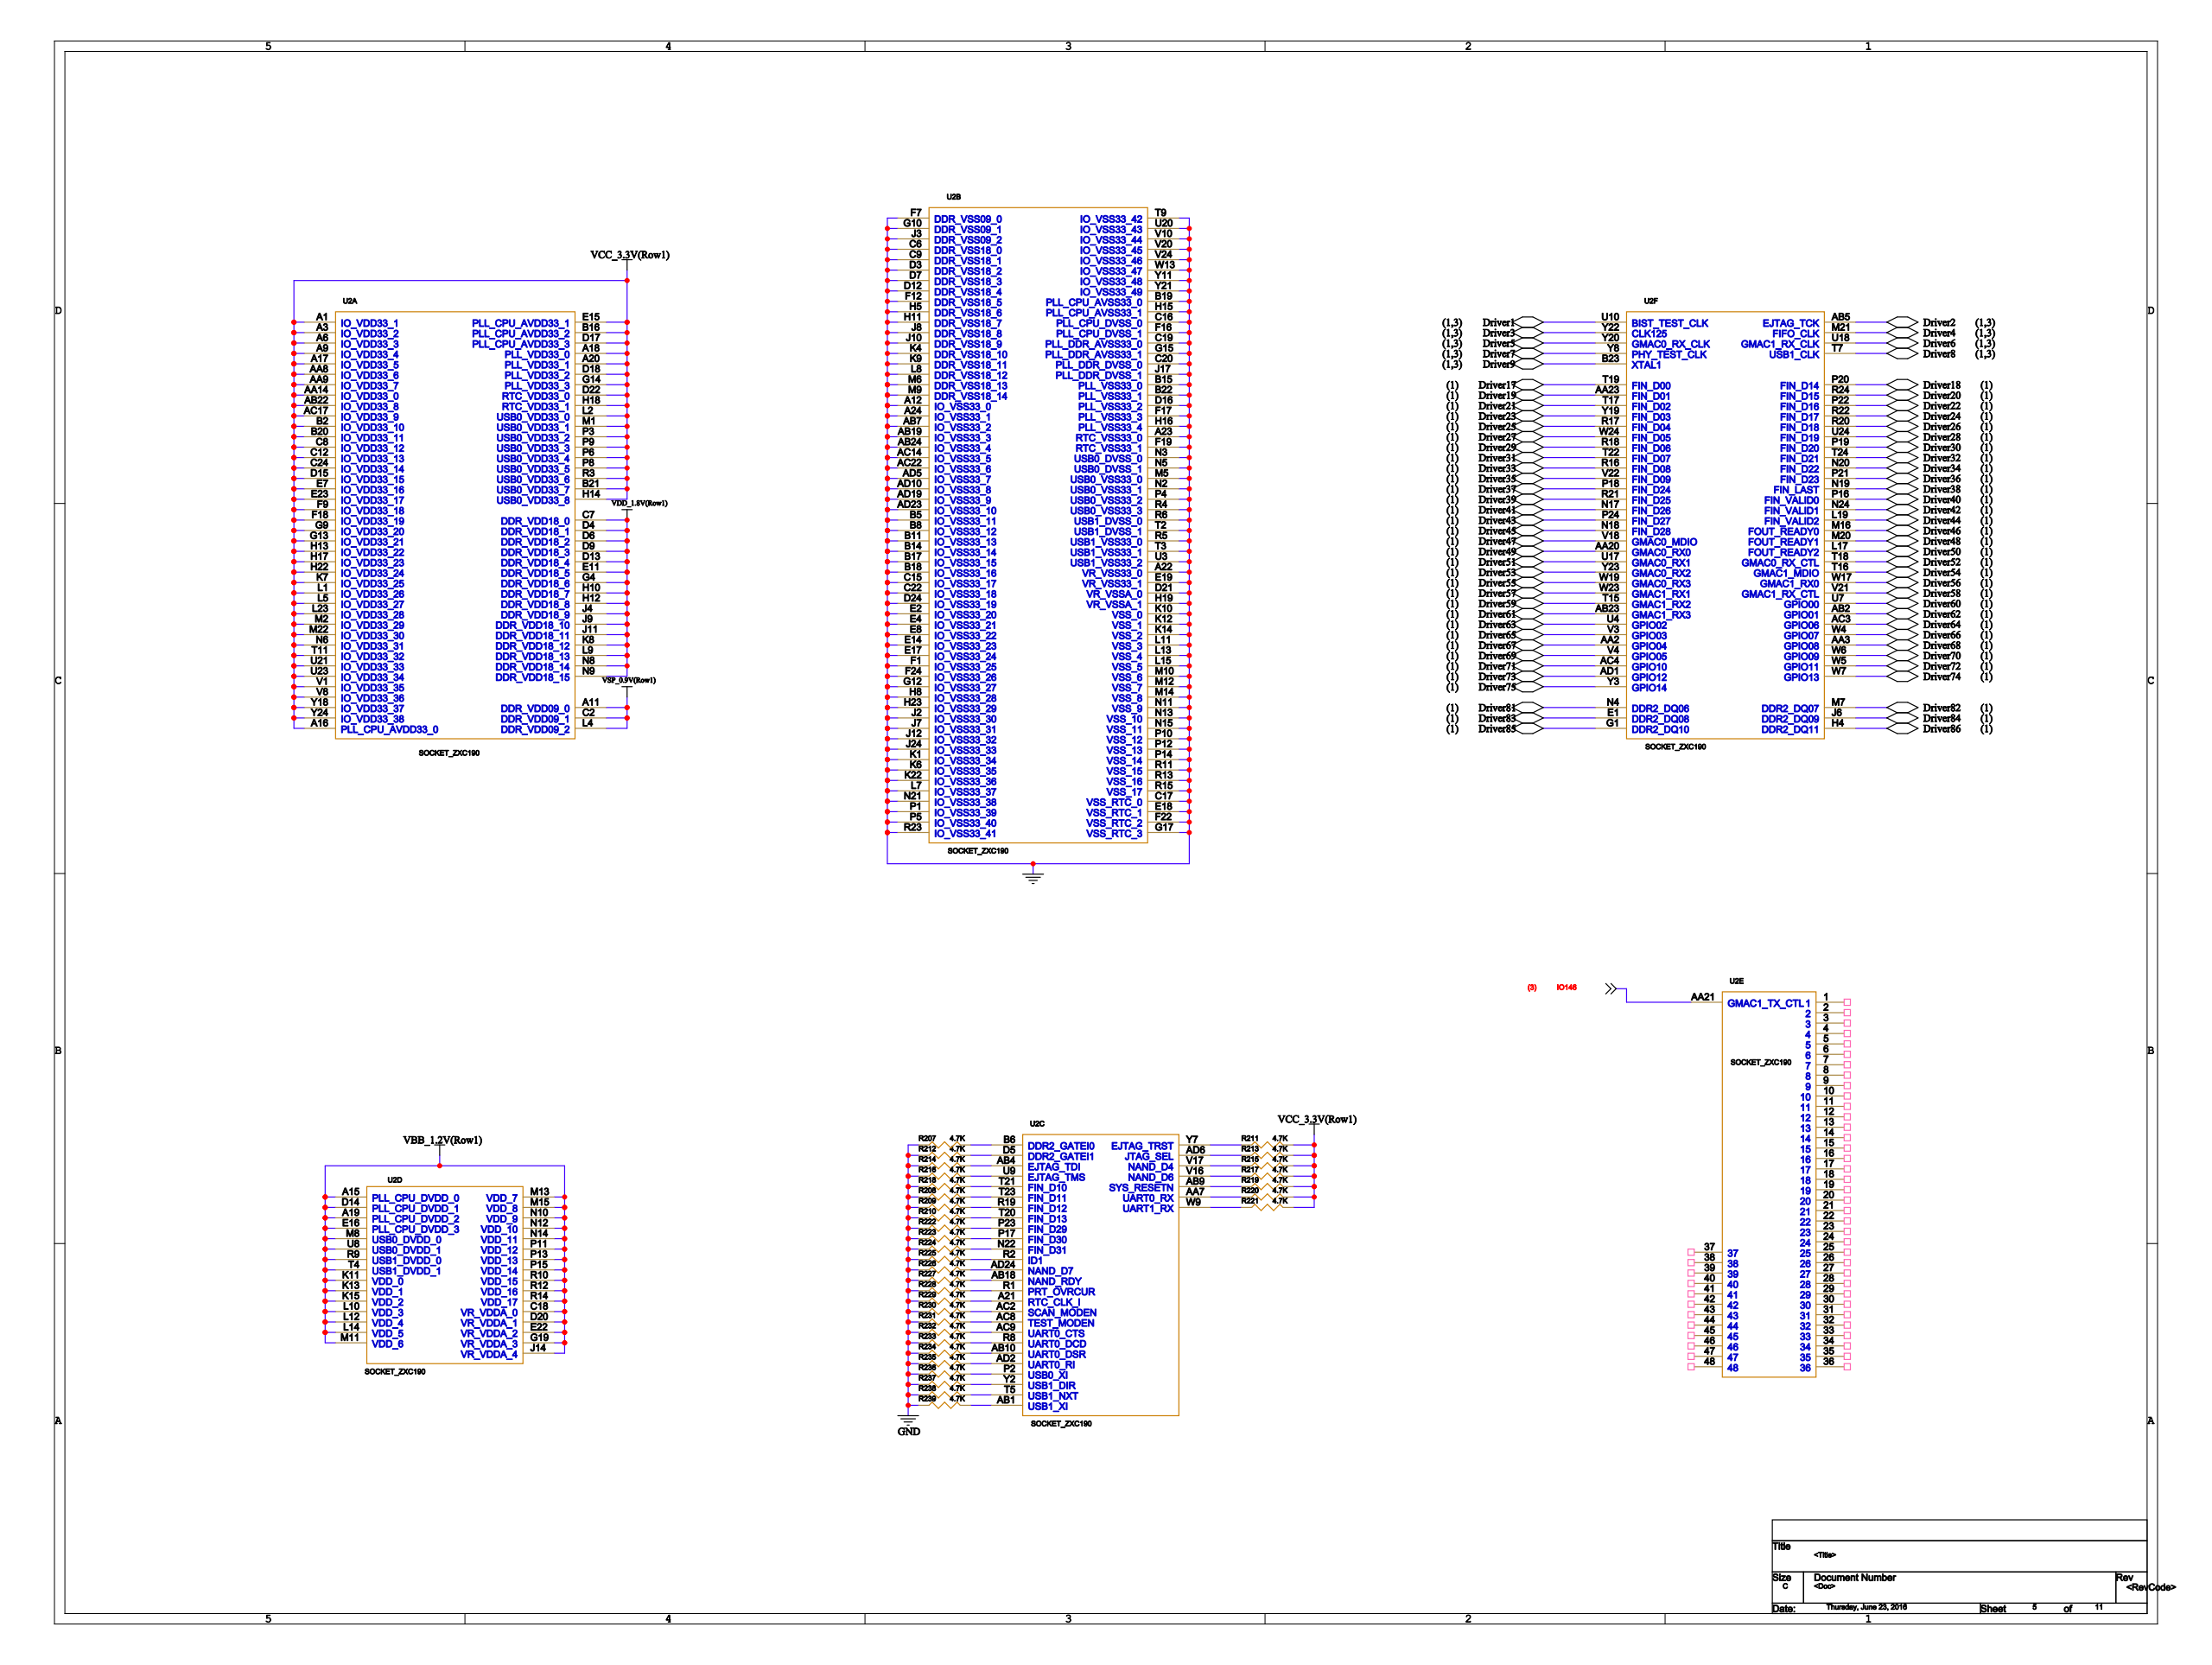Circuit board | Cadence Allegro | 531 parts | 624 nets | one sheet of the schematic
Parts on this sheet (reference | value | footprint):
R207 | 4.7K | R0805
R208 | 4.7K | R0805
R209 | 4.7K | R0805
R210 | 4.7K | R0805
R211 | 4.7K | R0805
R212 | 4.7K | R0805
R213 | 4.7K | R0805
R214 | 4.7K | R0805
R215 | 4.7K | R0805
R216 | 4.7K | R0805
R217 | 4.7K | R0805
R218 | 4.7K | R0805
R219 | 4.7K | R0805
R220 | 4.7K | R0805
R221 | 4.7K | R0805
R222 | 4.7K | R0805
R223 | 4.7K | R0805
R224 | 4.7K | R0805
R225 | 4.7K | R0805
R226 | 4.7K | R0805
R227 | 4.7K | R0805
R228 | 4.7K | R0805
R229 | 4.7K | R0805
R230 | 4.7K | R0805
R231 | 4.7K | R0805
R232 | 4.7K | R0805
R233 | 4.7K | R0805
R234 | 4.7K | R0805
R235 | 4.7K | R0805
R236 | 4.7K | R0805
R237 | 4.7K | R0805
R238 | 4.7K | R0805
R239 | 4.7K | R0805
U2 | SOCKET_ZXC190 | BGA-576
U3 | SOCKET_ZXC190 | BGA-576
U4 | SOCKET_ZXC190 | BGA-576
U10 | SOCKET_ZXC190 | BGA-576
Nets of these parts (net: part-pin ...):
GND: R207-1 R208-1 R209-1 R210-1 R212-1 R214-1 R216-1 R218-1 R222-1 R223-1 R224-1 R225-1 R226-1 R227-1 R228-1 R229-1 R230-1 R231-1 R232-1 R233-1 R234-1 R235-1 R236-1 R237-1 R238-1 R239-1 U2-A12 U2-A22 U2-A23 U2-A24 U2-AB7 U2-AB19 U2-AB24 U2-AC14 U2-AC22 U2-AD5 U2-AD10 U2-AD19 U2-AD23 U2-B5 U2-B8 U2-B11 U2-B14 U2-B15 U2-B17 U2-B18 U2-B19 U2-B22 U2-C6 U2-C9 U2-C15 U2-C16 U2-C17 U2-C19 U2-C20 U2-C22 U2-D3 U2-D7 U2-D12 U2-D16 U2-D21 U2-D24 U2-E2 U2-E4 U2-E8 U2-E14 U2-E17 U2-E18 U2-E19 U2-F1 U2-F7 U2-F12 U2-F16 U2-F17 U2-F19 U2-F22 U2-F24 U2-G10 U2-G12 U2-G15 U2-G17 U2-H5 U2-H8 U2-H11 U2-H15 U2-H16 U2-H19 U2-H23 U2-J2 U2-J3 U2-J7 U2-J8 U2-J10 U2-J12 U2-J17 U2-J24 U2-K1 U2-K4 U2-K6 U2-K9 U2-K10 U2-K12 U2-K14 U2-K22 U2-L7 U2-L8 U2-L11 U2-L13 U2-L15 U2-M5 U2-M6 U2-M9 U2-M10 U2-M12 U2-M14 U2-N2 U2-N3 U2-N5 U2-N11 U2-N13 U2-N15 U2-N21 U2-P1 U2-P4 U2-P5 U2-P10 U2-P12 U2-P14 U2-R4 U2-R5 U2-R6 U2-R11 U2-R13 U2-R15 U2-R23 U2-T2 U2-T3 U2-T9 U2-U3 U2-U20 U2-V10 U2-V20 U2-V24 U2-W13 U2-Y11 U2-Y21 U3-A12 U3-A22 U3-A23 U3-A24 U3-AB7 U3-AB19 U3-AB24 U3-AC14 U3-AC22 U3-AD5 U3-AD10 U3-AD19 U3-AD23 U3-B5 U3-B8 U3-B11 U3-B14 U3-B15 U3-B17 U3-B18 U3-B19 U3-B22 U3-C6 U3-C9 U3-C15 U3-C16 U3-C17 U3-C19 U3-C20 U3-C22 U3-D3 U3-D7 U3-D12 U3-D16 U3-D21 U3-D24 U3-E2 U3-E4 U3-E8 U3-E14 U3-E17 U3-E18 U3-E19 U3-F1 U3-F7 U3-F12 U3-F16 U3-F17 U3-F19 U3-F22 U3-F24 U3-G10 U3-G12 U3-G15 U3-G17 U3-H5 U3-H8 U3-H11 U3-H15 U3-H16 U3-H19 U3-H23 U3-J2 U3-J3 U3-J7 U3-J8 U3-J10 U3-J12 U3-J17 U3-J24 U3-K1 U3-K4 U3-K6 U3-K9 U3-K10 U3-K12 U3-K14 U3-K22 U3-L7 U3-L8 U3-L11 U3-L13 U3-L15 U3-M5 U3-M6 U3-M9 U3-M10 U3-M12 U3-M14 U3-N2 U3-N3 U3-N5 U3-N11 U3-N13 U3-N15 U3-N21 U3-P1 U3-P4 U3-P5 U3-P10 U3-P12 U3-P14 U3-R4 U3-R5 U3-R6 U3-R11 U3-R13 U3-R15 U3-R23 U3-T2 U3-T3 U3-T9 U3-U3 U3-U20 U3-V10 U3-V20 U3-V24 U3-W13 U3-Y11 U3-Y21 U4-A12 U4-A22 U4-A23 U4-A24 U4-AB7 U4-AB19 U4-AB24 U4-AC14 U4-AC22 U4-AD5 U4-AD10 U4-AD19 U4-AD23 U4-B5 U4-B8 U4-B11 U4-B14 U4-B15 U4-B17 U4-B18 U4-B19 U4-B22 U4-C6 U4-C9 U4-C15 U4-C16 U4-C17 U4-C19 U4-C20 U4-C22 U4-D3 U4-D7 U4-D12 U4-D16 U4-D21 U4-D24 U4-E2 U4-E4 U4-E8 U4-E14 U4-E17 U4-E18 U4-E19 U4-F1 U4-F7 U4-F12 U4-F16 U4-F17 U4-F19 U4-F22 U4-F24 U4-G10 U4-G12 U4-G15 U4-G17 U4-H5 U4-H8 U4-H11 U4-H15 U4-H16 U4-H19 U4-H23 U4-J2 U4-J3 U4-J7 U4-J8 U4-J10 U4-J12 U4-J17 U4-J24 U4-K1 U4-K4 U4-K6 U4-K9 U4-K10 U4-K12 U4-K14 U4-K22 U4-L7 U4-L8 U4-L11 U4-L13 U4-L15 U4-M5 U4-M6 U4-M9 U4-M10 U4-M12 U4-M14 U4-N2 U4-N3 U4-N5 U4-N11 U4-N13 U4-N15 U4-N21 U4-P1 U4-P4 U4-P5 U4-P10 U4-P12 U4-P14 U4-R4 U4-R5 U4-R6 U4-R11 U4-R13 U4-R15 U4-R23 U4-T2 U4-T3 U4-T9 U4-U3 U4-U20 U4-V10 U4-V20 U4-V24 U4-W13 U4-Y11 U4-Y21 U10-A12 U10-A22 U10-A23 U10-A24 U10-AB7 U10-AB19 U10-AB24 U10-AC14 U10-AC22 U10-AD5 U10-AD10 U10-AD19 U10-AD23 U10-B5 U10-B8 U10-B11 U10-B14 U10-B15 U10-B17 U10-B18 U10-B19 U10-B22 U10-C6 U10-C9 U10-C15 U10-C16 U10-C17 U10-C19 U10-C20 U10-C22 U10-D3 U10-D7 U10-D12 U10-D16 U10-D21 U10-D24 U10-E2 U10-E4 U10-E8 U10-E14 U10-E17 U10-E18 U10-E19 U10-F1 U10-F7 U10-F12 U10-F16 U10-F17 U10-F19 U10-F22 U10-F24 U10-G10 U10-G12 U10-G15 U10-G17 U10-H5 U10-H8 U10-H11 U10-H15 U10-H16 U10-H19 U10-H23 U10-J2 U10-J3 U10-J7 U10-J8 U10-J10 U10-J12 U10-J17 U10-J24 U10-K1 U10-K4 U10-K6 U10-K9 U10-K10 U10-K12 U10-K14 U10-K22 U10-L7 U10-L8 U10-L11 U10-L13 U10-L15 U10-M5 U10-M6 U10-M9 U10-M10 U10-M12 U10-M14 U10-N2 U10-N3 U10-N5 U10-N11 U10-N13 U10-N15 U10-N21 U10-P1 U10-P4 U10-P5 U10-P10 U10-P12 U10-P14 U10-R4 U10-R5 U10-R6 U10-R11 U10-R13 U10-R15 U10-R23 U10-T2 U10-T3 U10-T9 U10-U3 U10-U20 U10-V10 U10-V20 U10-V24 U10-W13 U10-Y11 U10-Y21
VCC_3.3V(ROW1): R211-2 R213-2 R215-2 R217-2 R219-2 R220-2 R221-2 U2-A1 U2-A3 U2-A6 U2-A9 U2-A16 U2-A17 U2-A18 U2-A20 U2-AA8 U2-AA9 U2-AA14 U2-AB22 U2-AC17 U2-B2 U2-B16 U2-B20 U2-B21 U2-C8 U2-C12 U2-C24 U2-D15 U2-D17 U2-D18 U2-D22 U2-E7 U2-E15 U2-E23 U2-F9 U2-F18 U2-G9 U2-G13 U2-G14 U2-H13 U2-H14 U2-H17 U2-H18 U2-H22 U2-K7 U2-L1 U2-L2 U2-L5 U2-L23 U2-M1 U2-M2 U2-M22 U2-N6 U2-P3 U2-P6 U2-P8 U2-P9 U2-R3 U2-T11 U2-U21 U2-U23 U2-V1 U2-V8 U2-Y18 U2-Y24 U3-A1 U3-A3 U3-A6 U3-A9 U3-A16 U3-A17 U3-A18 U3-A20 U3-AA8 U3-AA9 U3-AA14 U3-AB22 U3-AC17 U3-B2 U3-B16 U3-B20 U3-B21 U3-C8 U3-C12 U3-C24 U3-D15 U3-D17 U3-D18 U3-D22 U3-E7 U3-E15 U3-E23 U3-F9 U3-F18 U3-G9 U3-G13 U3-G14 U3-H13 U3-H14 U3-H17 U3-H18 U3-H22 U3-K7 U3-L1 U3-L2 U3-L5 U3-L23 U3-M1 U3-M2 U3-M22 U3-N6 U3-P3 U3-P6 U3-P8 U3-P9 U3-R3 U3-T11 U3-U21 U3-U23 U3-V1 U3-V8 U3-Y18 U3-Y24 U4-A1 U4-A3 U4-A6 U4-A9 U4-A16 U4-A17 U4-A18 U4-A20 U4-AA8 U4-AA9 U4-AA14 U4-AB22 U4-AC17 U4-B2 U4-B16 U4-B20 U4-B21 U4-C8 U4-C12 U4-C24 U4-D15 U4-D17 U4-D18 U4-D22 U4-E7 U4-E15 U4-E23 U4-F9 U4-F18 U4-G9 U4-G13 U4-G14 U4-H13 U4-H14 U4-H17 U4-H18 U4-H22 U4-K7 U4-L1 U4-L2 U4-L5 U4-L23 U4-M1 U4-M2 U4-M22 U4-N6 U4-P3 U4-P6 U4-P8 U4-P9 U4-R3 U4-T11 U4-U21 U4-U23 U4-V1 U4-V8 U4-Y18 U4-Y24
N8538231: R207-2 U2-B6
N8538211: R208-2 U2-T23
N8538207: R209-2 U2-R19
N8538263: R210-2 U2-T20
N8538655: R211-1 U2-Y7
N8538227: R212-2 U2-D5
N8538691: R213-1 U2-AD6
N8538223: R214-2 U2-AB4
N8538835: R215-1 U2-V17
N8538219: R216-2 U2-U9
N8538839: R217-1 U2-V16
N8538215: R218-2 U2-T21
N8538863: R219-1 U2-AB9
N8538843: R220-1 U2-AA7
N8538187: R221-1 U2-W9
N8538259: R222-2 U2-P23
N8538255: R223-2 U2-P17
N8538251: R224-2 U2-N22
N8538247: R225-2 U2-R2
N8538243: R226-2 U2-AD24
N8538239: R227-2 U2-AB18
N8538235: R228-2 U2-R1
N8538291: R229-2 U2-A21
N8538287: R230-2 U2-AC2
N8538283: R231-2 U2-AC8
N8538279: R232-2 U2-AC9
N8538727: R233-2 U2-R8
N8538275: R234-2 U2-AB10
N8538271: R235-2 U2-AD2
N8538267: R236-2 U2-P2
N8538303: R237-2 U2-Y2
N8538299: R238-2 U2-T5
N8538295: R239-2 U2-AB1
IO146: U2-AA21